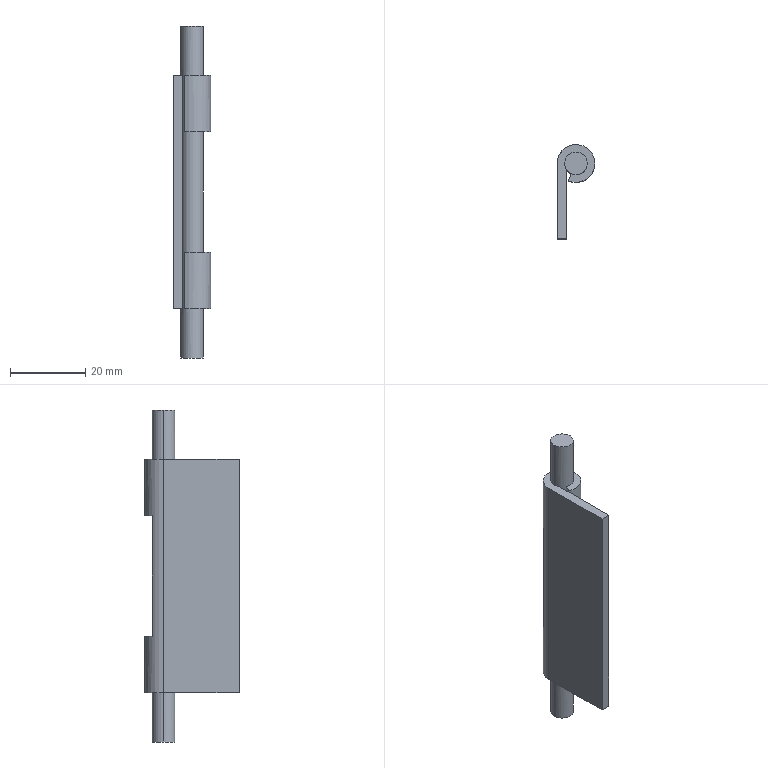Part | NX | features solid 2 | 1 solid | 17 faces | box 10 x 25 x 88 mm | volume 6948 mm3 | plane 12 | cylinder 5 | commonest cylinder face diameters 6 x4 10 x1
STEP:
#1=CARTESIAN_POINT('',(-1100.5,-763.,948.5));
#2=VERTEX_POINT('',#1);
#3=CARTESIAN_POINT('',(-1106.5,-763.,948.5));
#4=VERTEX_POINT('',#3);
#5=CARTESIAN_POINT('',(-1103.5,-763.,948.5));
#6=DIRECTION('',(0.,0.,-1.));
#7=DIRECTION('',(0.,1.,0.));
#8=AXIS2_PLACEMENT_3D('',#5,#6,#7);
#9=CIRCLE('',#8,3.);
#10=EDGE_CURVE('',#2,#4,#9,.T.);
#11=ORIENTED_EDGE('',*,*,#10,.F.);
#12=CARTESIAN_POINT('',(-1103.5,-763.,948.5));
#13=DIRECTION('',(0.,0.,-1.));
#14=DIRECTION('',(0.,1.,0.));
#15=AXIS2_PLACEMENT_3D('',#12,#13,#14);
#16=CIRCLE('',#15,3.);
#17=EDGE_CURVE('',#4,#2,#16,.T.);
#18=ORIENTED_EDGE('',*,*,#17,.F.);
#19=EDGE_LOOP('',(#11,#18));
#20=FACE_BOUND('',#19,.T.);
#21=CARTESIAN_POINT('',(-1103.5,-763.,948.5));
#22=DIRECTION('',(0.,0.,-1.));
#23=DIRECTION('',(0.,-1.,0.));
#24=AXIS2_PLACEMENT_3D('',#21,#22,#23);
#25=PLANE('',#24);
#26=ADVANCED_FACE('',(#20),#25,.F.);
#27=CARTESIAN_POINT('',(-1100.5,-763.,860.5));
#28=VERTEX_POINT('',#27);
#29=CARTESIAN_POINT('',(-1106.5,-763.,860.5));
#30=VERTEX_POINT('',#29);
#31=CARTESIAN_POINT('',(-1103.5,-763.,860.5));
#32=DIRECTION('',(0.,0.,-1.));
#33=DIRECTION('',(0.,1.,0.));
#34=AXIS2_PLACEMENT_3D('',#31,#32,#33);
#35=CIRCLE('',#34,3.);
#36=EDGE_CURVE('',#28,#30,#35,.T.);
#37=ORIENTED_EDGE('',*,*,#36,.T.);
#38=CARTESIAN_POINT('',(-1103.5,-763.,860.5));
#39=DIRECTION('',(0.,0.,-1.));
#40=DIRECTION('',(0.,1.,0.));
#41=AXIS2_PLACEMENT_3D('',#38,#39,#40);
#42=CIRCLE('',#41,3.);
#43=EDGE_CURVE('',#30,#28,#42,.T.);
#44=ORIENTED_EDGE('',*,*,#43,.T.);
#45=EDGE_LOOP('',(#37,#44));
#46=FACE_BOUND('',#45,.T.);
#47=CARTESIAN_POINT('',(-1103.5,-763.,860.5));
#48=DIRECTION('',(0.,0.,-1.));
#49=DIRECTION('',(0.,-1.,0.));
#50=AXIS2_PLACEMENT_3D('',#47,#48,#49);
#51=PLANE('',#50);
#52=ADVANCED_FACE('',(#46),#51,.T.);
#53=CARTESIAN_POINT('',(-1100.5,-763.,888.5));
#54=VERTEX_POINT('',#53);
#55=CARTESIAN_POINT('',(-1100.5,-763.,920.5));
#56=VERTEX_POINT('',#55);
#57=CARTESIAN_POINT('',(-1100.5,-763.,860.5));
#58=DIRECTION('',(0.,0.,1.));
#59=VECTOR('',#58,1000.);
#60=LINE('',#57,#59);
#61=EDGE_CURVE('',#54,#56,#60,.T.);
#62=ORIENTED_EDGE('',*,*,#61,.F.);
#63=CARTESIAN_POINT('',(-1105.9,-761.2,888.5));
#64=VERTEX_POINT('',#63);
#65=CARTESIAN_POINT('',(-1103.5,-763.,888.5));
#66=DIRECTION('',(0.,0.,1.));
#67=DIRECTION('',(1.,0.,0.));
#68=AXIS2_PLACEMENT_3D('',#65,#66,#67);
#69=CIRCLE('',#68,3.);
#70=EDGE_CURVE('',#54,#64,#69,.T.);
#71=ORIENTED_EDGE('',*,*,#70,.T.);
#72=CARTESIAN_POINT('',(-1105.9,-761.2,920.5));
#73=VERTEX_POINT('',#72);
#74=CARTESIAN_POINT('',(-1105.9,-761.2,860.5));
#75=DIRECTION('',(0.,0.,1.));
#76=VECTOR('',#75,1000.);
#77=LINE('',#74,#76);
#78=EDGE_CURVE('',#64,#73,#77,.T.);
#79=ORIENTED_EDGE('',*,*,#78,.T.);
#80=CARTESIAN_POINT('',(-1103.5,-763.,920.5));
#81=DIRECTION('',(0.,0.,-1.));
#82=DIRECTION('',(-1.,0.,0.));
#83=AXIS2_PLACEMENT_3D('',#80,#81,#82);
#84=CIRCLE('',#83,3.);
#85=EDGE_CURVE('',#73,#56,#84,.T.);
#86=ORIENTED_EDGE('',*,*,#85,.T.);
#87=EDGE_LOOP('',(#62,#71,#79,#86));
#88=FACE_BOUND('',#87,.T.);
#89=CARTESIAN_POINT('',(-1103.5,-763.,860.5));
#90=DIRECTION('',(0.,0.,1.));
#91=DIRECTION('',(1.,0.,0.));
#92=AXIS2_PLACEMENT_3D('',#89,#90,#91);
#93=CYLINDRICAL_SURFACE('',#92,3.);
#94=ADVANCED_FACE('',(#88),#93,.T.);
#95=CARTESIAN_POINT('',(-1106.,-783.,935.5));
#96=VERTEX_POINT('',#95);
#97=CARTESIAN_POINT('',(-1106.,-783.,873.5));
#98=VERTEX_POINT('',#97);
#99=CARTESIAN_POINT('',(-1106.,-783.,935.5));
#100=DIRECTION('',(0.,0.,-1.));
#101=VECTOR('',#100,1000.);
#102=LINE('',#99,#101);
#103=EDGE_CURVE('',#96,#98,#102,.T.);
#104=ORIENTED_EDGE('',*,*,#103,.F.);
#105=CARTESIAN_POINT('',(-1108.5,-783.,935.5));
#106=VERTEX_POINT('',#105);
#107=CARTESIAN_POINT('',(-1108.5,-783.,935.5));
#108=DIRECTION('',(-1.,0.,0.));
#109=VECTOR('',#108,1000.);
#110=LINE('',#107,#109);
#111=EDGE_CURVE('',#96,#106,#110,.T.);
#112=ORIENTED_EDGE('',*,*,#111,.T.);
#113=CARTESIAN_POINT('',(-1108.5,-783.,873.5));
#114=VERTEX_POINT('',#113);
#115=CARTESIAN_POINT('',(-1108.5,-783.,935.5));
#116=DIRECTION('',(0.,0.,-1.));
#117=VECTOR('',#116,1000.);
#118=LINE('',#115,#117);
#119=EDGE_CURVE('',#106,#114,#118,.T.);
#120=ORIENTED_EDGE('',*,*,#119,.T.);
#121=CARTESIAN_POINT('',(-1108.5,-783.,873.5));
#122=DIRECTION('',(-1.,0.,0.));
#123=VECTOR('',#122,1000.);
#124=LINE('',#121,#123);
#125=EDGE_CURVE('',#98,#114,#124,.T.);
#126=ORIENTED_EDGE('',*,*,#125,.F.);
#127=EDGE_LOOP('',(#104,#112,#120,#126));
#128=FACE_BOUND('',#127,.T.);
#129=CARTESIAN_POINT('',(-1108.5,-783.,935.5));
#130=DIRECTION('',(0.,1.,0.));
#131=DIRECTION('',(0.,0.,-1.));
#132=AXIS2_PLACEMENT_3D('',#129,#130,#131);
#133=PLANE('',#132);
#134=ADVANCED_FACE('',(#128),#133,.F.);
#135=CARTESIAN_POINT('',(-1105.5,-767.583,888.5));
#136=VERTEX_POINT('',#135);
#137=CARTESIAN_POINT('',(-1107.5,-760.,888.5));
#138=VERTEX_POINT('',#137);
#139=CARTESIAN_POINT('',(-1103.5,-763.,888.5));
#140=DIRECTION('',(0.,0.,1.));
#141=DIRECTION('',(-1.,0.,0.));
#142=AXIS2_PLACEMENT_3D('',#139,#140,#141);
#143=CIRCLE('',#142,5.);
#144=EDGE_CURVE('',#136,#138,#143,.T.);
#145=ORIENTED_EDGE('',*,*,#144,.F.);
#146=CARTESIAN_POINT('',(-1105.5,-767.583,873.5));
#147=VERTEX_POINT('',#146);
#148=CARTESIAN_POINT('',(-1105.5,-767.583,935.5));
#149=DIRECTION('',(0.,0.,-1.));
#150=VECTOR('',#149,1000.);
#151=LINE('',#148,#150);
#152=EDGE_CURVE('',#136,#147,#151,.T.);
#153=ORIENTED_EDGE('',*,*,#152,.T.);
#154=CARTESIAN_POINT('',(-1108.5,-763.,873.5));
#155=VERTEX_POINT('',#154);
#156=CARTESIAN_POINT('',(-1103.5,-763.,873.5));
#157=DIRECTION('',(0.,0.,-1.));
#158=DIRECTION('',(-1.,0.,0.));
#159=AXIS2_PLACEMENT_3D('',#156,#157,#158);
#160=CIRCLE('',#159,5.);
#161=EDGE_CURVE('',#155,#147,#160,.T.);
#162=ORIENTED_EDGE('',*,*,#161,.F.);
#163=CARTESIAN_POINT('',(-1108.5,-763.,935.5));
#164=VERTEX_POINT('',#163);
#165=CARTESIAN_POINT('',(-1108.5,-763.,935.5));
#166=DIRECTION('',(0.,0.,-1.));
#167=VECTOR('',#166,1000.);
#168=LINE('',#165,#167);
#169=EDGE_CURVE('',#164,#155,#168,.T.);
#170=ORIENTED_EDGE('',*,*,#169,.F.);
#171=CARTESIAN_POINT('',(-1105.5,-767.583,935.5));
#172=VERTEX_POINT('',#171);
#173=CARTESIAN_POINT('',(-1103.5,-763.,935.5));
#174=DIRECTION('',(0.,0.,-1.));
#175=DIRECTION('',(-1.,0.,0.));
#176=AXIS2_PLACEMENT_3D('',#173,#174,#175);
#177=CIRCLE('',#176,5.);
#178=EDGE_CURVE('',#164,#172,#177,.T.);
#179=ORIENTED_EDGE('',*,*,#178,.T.);
#180=CARTESIAN_POINT('',(-1105.5,-767.583,920.5));
#181=VERTEX_POINT('',#180);
#182=CARTESIAN_POINT('',(-1105.5,-767.583,935.5));
#183=DIRECTION('',(0.,0.,-1.));
#184=VECTOR('',#183,1000.);
#185=LINE('',#182,#184);
#186=EDGE_CURVE('',#172,#181,#185,.T.);
#187=ORIENTED_EDGE('',*,*,#186,.T.);
#188=CARTESIAN_POINT('',(-1107.5,-760.,920.5));
#189=VERTEX_POINT('',#188);
#190=CARTESIAN_POINT('',(-1103.5,-763.,920.5));
#191=DIRECTION('',(0.,0.,-1.));
#192=DIRECTION('',(1.,0.,0.));
#193=AXIS2_PLACEMENT_3D('',#190,#191,#192);
#194=CIRCLE('',#193,5.);
#195=EDGE_CURVE('',#189,#181,#194,.T.);
#196=ORIENTED_EDGE('',*,*,#195,.F.);
#197=CARTESIAN_POINT('',(-1107.5,-760.,935.5));
#198=DIRECTION('',(0.,0.,1.));
#199=VECTOR('',#198,1000.);
#200=LINE('',#197,#199);
#201=EDGE_CURVE('',#138,#189,#200,.T.);
#202=ORIENTED_EDGE('',*,*,#201,.F.);
#203=EDGE_LOOP('',(#145,#153,#162,#170,#179,#187,#196,#202));
#204=FACE_BOUND('',#203,.T.);
#205=CARTESIAN_POINT('',(-1103.5,-763.,935.5));
#206=DIRECTION('',(0.,0.,-1.));
#207=DIRECTION('',(-1.,0.,0.));
#208=AXIS2_PLACEMENT_3D('',#205,#206,#207);
#209=CYLINDRICAL_SURFACE('',#208,5.);
#210=ADVANCED_FACE('',(#204),#209,.T.);
#211=CARTESIAN_POINT('',(-1108.5,-783.,873.5));
#212=DIRECTION('',(0.,1.,0.));
#213=VECTOR('',#212,1000.);
#214=LINE('',#211,#213);
#215=EDGE_CURVE('',#114,#155,#214,.T.);
#216=ORIENTED_EDGE('',*,*,#215,.F.);
#217=ORIENTED_EDGE('',*,*,#119,.F.);
#218=CARTESIAN_POINT('',(-1108.5,-783.,935.5));
#219=DIRECTION('',(0.,1.,0.));
#220=VECTOR('',#219,1000.);
#221=LINE('',#218,#220);
#222=EDGE_CURVE('',#106,#164,#221,.T.);
#223=ORIENTED_EDGE('',*,*,#222,.T.);
#224=ORIENTED_EDGE('',*,*,#169,.T.);
#225=EDGE_LOOP('',(#216,#217,#223,#224));
#226=FACE_BOUND('',#225,.T.);
#227=CARTESIAN_POINT('',(-1108.5,-783.,935.5));
#228=DIRECTION('',(-1.,0.,0.));
#229=DIRECTION('',(0.,1.,0.));
#230=AXIS2_PLACEMENT_3D('',#227,#228,#229);
#231=PLANE('',#230);
#232=ADVANCED_FACE('',(#226),#231,.T.);
#233=ORIENTED_EDGE('',*,*,#78,.F.);
#234=CARTESIAN_POINT('',(-1105.5,-761.5,888.5));
#235=DIRECTION('',(0.8,-0.6,0.));
#236=VECTOR('',#235,1000.);
#237=LINE('',#234,#236);
#238=EDGE_CURVE('',#138,#64,#237,.T.);
#239=ORIENTED_EDGE('',*,*,#238,.F.);
#240=ORIENTED_EDGE('',*,*,#201,.T.);
#241=CARTESIAN_POINT('',(-1105.5,-761.5,920.5));
#242=DIRECTION('',(0.8,-0.6,0.));
#243=VECTOR('',#242,1000.);
#244=LINE('',#241,#243);
#245=EDGE_CURVE('',#189,#73,#244,.T.);
#246=ORIENTED_EDGE('',*,*,#245,.T.);
#247=EDGE_LOOP('',(#233,#239,#240,#246));
#248=FACE_BOUND('',#247,.T.);
#249=CARTESIAN_POINT('',(-1105.5,-761.5,904.5));
#250=DIRECTION('',(0.6,0.8,0.));
#251=DIRECTION('',(0.,0.,-1.));
#252=AXIS2_PLACEMENT_3D('',#249,#250,#251);
#253=PLANE('',#252);
#254=ADVANCED_FACE('',(#248),#253,.T.);
#255=ORIENTED_EDGE('',*,*,#85,.F.);
#256=ORIENTED_EDGE('',*,*,#245,.F.);
#257=ORIENTED_EDGE('',*,*,#195,.T.);
#258=CARTESIAN_POINT('',(-1104.7,-765.75,920.5));
#259=VERTEX_POINT('',#258);
#260=CARTESIAN_POINT('',(-1105.5,-767.583,920.5));
#261=DIRECTION('',(-0.4,-0.9165,0.));
#262=VECTOR('',#261,1000.);
#263=LINE('',#260,#262);
#264=EDGE_CURVE('',#259,#181,#263,.T.);
#265=ORIENTED_EDGE('',*,*,#264,.F.);
#266=CARTESIAN_POINT('',(-1103.5,-763.,920.5));
#267=DIRECTION('',(0.,0.,-1.));
#268=DIRECTION('',(-1.,0.,0.));
#269=AXIS2_PLACEMENT_3D('',#266,#267,#268);
#270=CIRCLE('',#269,3.);
#271=EDGE_CURVE('',#56,#259,#270,.T.);
#272=ORIENTED_EDGE('',*,*,#271,.F.);
#273=EDGE_LOOP('',(#255,#256,#257,#265,#272));
#274=FACE_BOUND('',#273,.T.);
#275=CARTESIAN_POINT('',(-1103.5,-763.,920.5));
#276=DIRECTION('',(0.,0.,-1.));
#277=DIRECTION('',(0.,-1.,0.));
#278=AXIS2_PLACEMENT_3D('',#275,#276,#277);
#279=PLANE('',#278);
#280=ADVANCED_FACE('',(#274),#279,.T.);
#281=CARTESIAN_POINT('',(-1104.7,-765.75,888.5));
#282=VERTEX_POINT('',#281);
#283=CARTESIAN_POINT('',(-1103.5,-763.,888.5));
#284=DIRECTION('',(0.,0.,1.));
#285=DIRECTION('',(1.,0.,0.));
#286=AXIS2_PLACEMENT_3D('',#283,#284,#285);
#287=CIRCLE('',#286,3.);
#288=EDGE_CURVE('',#282,#54,#287,.T.);
#289=ORIENTED_EDGE('',*,*,#288,.F.);
#290=CARTESIAN_POINT('',(-1105.5,-767.583,888.5));
#291=DIRECTION('',(-0.4,-0.9165,0.));
#292=VECTOR('',#291,1000.);
#293=LINE('',#290,#292);
#294=EDGE_CURVE('',#282,#136,#293,.T.);
#295=ORIENTED_EDGE('',*,*,#294,.T.);
#296=ORIENTED_EDGE('',*,*,#144,.T.);
#297=ORIENTED_EDGE('',*,*,#238,.T.);
#298=ORIENTED_EDGE('',*,*,#70,.F.);
#299=EDGE_LOOP('',(#289,#295,#296,#297,#298));
#300=FACE_BOUND('',#299,.T.);
#301=CARTESIAN_POINT('',(-1103.5,-763.,888.5));
#302=DIRECTION('',(0.,0.,1.));
#303=DIRECTION('',(0.,-1.,0.));
#304=AXIS2_PLACEMENT_3D('',#301,#302,#303);
#305=PLANE('',#304);
#306=ADVANCED_FACE('',(#300),#305,.T.);
#307=CARTESIAN_POINT('',(-1106.,-764.658,935.5));
#308=VERTEX_POINT('',#307);
#309=CARTESIAN_POINT('',(-1106.,-764.658,873.5));
#310=VERTEX_POINT('',#309);
#311=CARTESIAN_POINT('',(-1106.,-764.658,860.5));
#312=DIRECTION('',(0.,0.,-1.));
#313=VECTOR('',#312,1000.);
#314=LINE('',#311,#313);
#315=EDGE_CURVE('',#308,#310,#314,.T.);
#316=ORIENTED_EDGE('',*,*,#315,.F.);
#317=CARTESIAN_POINT('',(-1106.,-783.,935.5));
#318=DIRECTION('',(0.,1.,0.));
#319=VECTOR('',#318,1000.);
#320=LINE('',#317,#319);
#321=EDGE_CURVE('',#96,#308,#320,.T.);
#322=ORIENTED_EDGE('',*,*,#321,.F.);
#323=ORIENTED_EDGE('',*,*,#103,.T.);
#324=CARTESIAN_POINT('',(-1106.,-783.,873.5));
#325=DIRECTION('',(0.,1.,0.));
#326=VECTOR('',#325,1000.);
#327=LINE('',#324,#326);
#328=EDGE_CURVE('',#98,#310,#327,.T.);
#329=ORIENTED_EDGE('',*,*,#328,.T.);
#330=EDGE_LOOP('',(#316,#322,#323,#329));
#331=FACE_BOUND('',#330,.T.);
#332=CARTESIAN_POINT('',(-1106.,-783.,935.5));
#333=DIRECTION('',(-1.,0.,0.));
#334=DIRECTION('',(0.,1.,0.));
#335=AXIS2_PLACEMENT_3D('',#332,#333,#334);
#336=PLANE('',#335);
#337=ADVANCED_FACE('',(#331),#336,.F.);
#338=CARTESIAN_POINT('',(-1104.7,-765.75,873.5));
#339=VERTEX_POINT('',#338);
#340=CARTESIAN_POINT('',(-1105.5,-767.583,873.5));
#341=DIRECTION('',(-0.4,-0.9165,0.));
#342=VECTOR('',#341,1000.);
#343=LINE('',#340,#342);
#344=EDGE_CURVE('',#339,#147,#343,.T.);
#345=ORIENTED_EDGE('',*,*,#344,.F.);
#346=CARTESIAN_POINT('',(-1100.5,-763.,873.5));
#347=VERTEX_POINT('',#346);
#348=CARTESIAN_POINT('',(-1103.5,-763.,873.5));
#349=DIRECTION('',(0.,0.,1.));
#350=DIRECTION('',(0.,-1.,0.));
#351=AXIS2_PLACEMENT_3D('',#348,#349,#350);
#352=CIRCLE('',#351,3.);
#353=EDGE_CURVE('',#339,#347,#352,.T.);
#354=ORIENTED_EDGE('',*,*,#353,.T.);
#355=CARTESIAN_POINT('',(-1106.5,-763.,873.5));
#356=VERTEX_POINT('',#355);
#357=CARTESIAN_POINT('',(-1103.5,-763.,873.5));
#358=DIRECTION('',(0.,0.,1.));
#359=DIRECTION('',(0.,-1.,0.));
#360=AXIS2_PLACEMENT_3D('',#357,#358,#359);
#361=CIRCLE('',#360,3.);
#362=EDGE_CURVE('',#347,#356,#361,.T.);
#363=ORIENTED_EDGE('',*,*,#362,.T.);
#364=CARTESIAN_POINT('',(-1103.5,-763.,873.5));
#365=DIRECTION('',(0.,0.,1.));
#366=DIRECTION('',(0.,-1.,0.));
#367=AXIS2_PLACEMENT_3D('',#364,#365,#366);
#368=CIRCLE('',#367,3.);
#369=EDGE_CURVE('',#356,#310,#368,.T.);
#370=ORIENTED_EDGE('',*,*,#369,.T.);
#371=ORIENTED_EDGE('',*,*,#328,.F.);
#372=ORIENTED_EDGE('',*,*,#125,.T.);
#373=ORIENTED_EDGE('',*,*,#215,.T.);
#374=ORIENTED_EDGE('',*,*,#161,.T.);
#375=EDGE_LOOP('',(#345,#354,#363,#370,#371,#372,#373,#374));
#376=FACE_BOUND('',#375,.T.);
#377=CARTESIAN_POINT('',(-1108.5,-783.,873.5));
#378=DIRECTION('',(0.,0.,1.));
#379=DIRECTION('',(0.,-1.,0.));
#380=AXIS2_PLACEMENT_3D('',#377,#378,#379);
#381=PLANE('',#380);
#382=ADVANCED_FACE('',(#376),#381,.F.);
#383=ORIENTED_EDGE('',*,*,#294,.F.);
#384=CARTESIAN_POINT('',(-1104.7,-765.75,860.5));
#385=DIRECTION('',(0.,0.,-1.));
#386=VECTOR('',#385,1000.);
#387=LINE('',#384,#386);
#388=EDGE_CURVE('',#282,#339,#387,.T.);
#389=ORIENTED_EDGE('',*,*,#388,.T.);
#390=ORIENTED_EDGE('',*,*,#344,.T.);
#391=ORIENTED_EDGE('',*,*,#152,.F.);
#392=EDGE_LOOP('',(#383,#389,#390,#391));
#393=FACE_BOUND('',#392,.T.);
#394=CARTESIAN_POINT('',(-1105.5,-767.583,904.5));
#395=DIRECTION('',(-0.9165,0.4,0.));
#396=DIRECTION('',(0.,0.,1.));
#397=AXIS2_PLACEMENT_3D('',#394,#395,#396);
#398=PLANE('',#397);
#399=ADVANCED_FACE('',(#393),#398,.T.);
#400=ORIENTED_EDGE('',*,*,#321,.T.);
#401=CARTESIAN_POINT('',(-1106.5,-763.,935.5));
#402=VERTEX_POINT('',#401);
#403=CARTESIAN_POINT('',(-1103.5,-763.,935.5));
#404=DIRECTION('',(0.,0.,-1.));
#405=DIRECTION('',(0.,-1.,0.));
#406=AXIS2_PLACEMENT_3D('',#403,#404,#405);
#407=CIRCLE('',#406,3.);
#408=EDGE_CURVE('',#308,#402,#407,.T.);
#409=ORIENTED_EDGE('',*,*,#408,.T.);
#410=CARTESIAN_POINT('',(-1100.5,-763.,935.5));
#411=VERTEX_POINT('',#410);
#412=CARTESIAN_POINT('',(-1103.5,-763.,935.5));
#413=DIRECTION('',(0.,0.,-1.));
#414=DIRECTION('',(0.,-1.,0.));
#415=AXIS2_PLACEMENT_3D('',#412,#413,#414);
#416=CIRCLE('',#415,3.);
#417=EDGE_CURVE('',#402,#411,#416,.T.);
#418=ORIENTED_EDGE('',*,*,#417,.T.);
#419=CARTESIAN_POINT('',(-1104.7,-765.75,935.5));
#420=VERTEX_POINT('',#419);
#421=CARTESIAN_POINT('',(-1103.5,-763.,935.5));
#422=DIRECTION('',(0.,0.,-1.));
#423=DIRECTION('',(0.,-1.,0.));
#424=AXIS2_PLACEMENT_3D('',#421,#422,#423);
#425=CIRCLE('',#424,3.);
#426=EDGE_CURVE('',#411,#420,#425,.T.);
#427=ORIENTED_EDGE('',*,*,#426,.T.);
#428=CARTESIAN_POINT('',(-1105.5,-767.583,935.5));
#429=DIRECTION('',(-0.4,-0.9165,0.));
#430=VECTOR('',#429,1000.);
#431=LINE('',#428,#430);
#432=EDGE_CURVE('',#420,#172,#431,.T.);
#433=ORIENTED_EDGE('',*,*,#432,.T.);
#434=ORIENTED_EDGE('',*,*,#178,.F.);
#435=ORIENTED_EDGE('',*,*,#222,.F.);
#436=ORIENTED_EDGE('',*,*,#111,.F.);
#437=EDGE_LOOP('',(#400,#409,#418,#427,#433,#434,#435,#436));
#438=FACE_BOUND('',#437,.T.);
#439=CARTESIAN_POINT('',(-1103.5,-763.,935.5));
#440=DIRECTION('',(0.,0.,1.));
#441=DIRECTION('',(0.,-1.,0.));
#442=AXIS2_PLACEMENT_3D('',#439,#440,#441);
#443=PLANE('',#442);
#444=ADVANCED_FACE('',(#438),#443,.T.);
#445=ORIENTED_EDGE('',*,*,#432,.F.);
#446=CARTESIAN_POINT('',(-1104.7,-765.75,860.5));
#447=DIRECTION('',(0.,0.,-1.));
#448=VECTOR('',#447,1000.);
#449=LINE('',#446,#448);
#450=EDGE_CURVE('',#420,#259,#449,.T.);
#451=ORIENTED_EDGE('',*,*,#450,.T.);
#452=ORIENTED_EDGE('',*,*,#264,.T.);
#453=ORIENTED_EDGE('',*,*,#186,.F.);
#454=EDGE_LOOP('',(#445,#451,#452,#453));
#455=FACE_BOUND('',#454,.T.);
#456=CARTESIAN_POINT('',(-1105.5,-767.583,904.5));
#457=DIRECTION('',(-0.9165,0.4,0.));
#458=DIRECTION('',(0.,0.,1.));
#459=AXIS2_PLACEMENT_3D('',#456,#457,#458);
#460=PLANE('',#459);
#461=ADVANCED_FACE('',(#455),#460,.T.);
#462=CARTESIAN_POINT('',(-1106.5,-763.,860.5));
#463=DIRECTION('',(0.,0.,1.));
#464=VECTOR('',#463,1000.);
#465=LINE('',#462,#464);
#466=EDGE_CURVE('',#30,#356,#465,.T.);
#467=ORIENTED_EDGE('',*,*,#466,.F.);
#468=ORIENTED_EDGE('',*,*,#36,.F.);
#469=CARTESIAN_POINT('',(-1100.5,-763.,860.5));
#470=DIRECTION('',(0.,0.,1.));
#471=VECTOR('',#470,1000.);
#472=LINE('',#469,#471);
#473=EDGE_CURVE('',#347,#28,#472,.F.);
#474=ORIENTED_EDGE('',*,*,#473,.F.);
#475=ORIENTED_EDGE('',*,*,#353,.F.);
#476=ORIENTED_EDGE('',*,*,#388,.F.);
#477=ORIENTED_EDGE('',*,*,#288,.T.);
#478=ORIENTED_EDGE('',*,*,#61,.T.);
#479=ORIENTED_EDGE('',*,*,#271,.T.);
#480=ORIENTED_EDGE('',*,*,#450,.F.);
#481=ORIENTED_EDGE('',*,*,#426,.F.);
#482=CARTESIAN_POINT('',(-1100.5,-763.,860.5));
#483=DIRECTION('',(0.,0.,1.));
#484=VECTOR('',#483,1000.);
#485=LINE('',#482,#484);
#486=EDGE_CURVE('',#2,#411,#485,.F.);
#487=ORIENTED_EDGE('',*,*,#486,.F.);
#488=ORIENTED_EDGE('',*,*,#10,.T.);
#489=CARTESIAN_POINT('',(-1106.5,-763.,860.5));
#490=DIRECTION('',(0.,0.,1.));
#491=VECTOR('',#490,1000.);
#492=LINE('',#489,#491);
#493=EDGE_CURVE('',#402,#4,#492,.T.);
#494=ORIENTED_EDGE('',*,*,#493,.F.);
#495=ORIENTED_EDGE('',*,*,#408,.F.);
#496=ORIENTED_EDGE('',*,*,#315,.T.);
#497=ORIENTED_EDGE('',*,*,#369,.F.);
#498=EDGE_LOOP('',(#467,#468,#474,#475,#476,#477,#478,#479,#480,#481,#487,#488,#494,#495,#496,#497));
#499=FACE_BOUND('',#498,.T.);
#500=CARTESIAN_POINT('',(-1103.5,-763.,860.5));
#501=DIRECTION('',(0.,0.,1.));
#502=DIRECTION('',(1.,0.,0.));
#503=AXIS2_PLACEMENT_3D('',#500,#501,#502);
#504=CYLINDRICAL_SURFACE('',#503,3.);
#505=ADVANCED_FACE('',(#499),#504,.T.);
#506=ORIENTED_EDGE('',*,*,#417,.F.);
#507=ORIENTED_EDGE('',*,*,#493,.T.);
#508=ORIENTED_EDGE('',*,*,#17,.T.);
#509=ORIENTED_EDGE('',*,*,#486,.T.);
#510=EDGE_LOOP('',(#506,#507,#508,#509));
#511=FACE_BOUND('',#510,.T.);
#512=CARTESIAN_POINT('',(-1103.5,-763.,860.5));
#513=DIRECTION('',(0.,0.,1.));
#514=DIRECTION('',(1.,0.,0.));
#515=AXIS2_PLACEMENT_3D('',#512,#513,#514);
#516=CYLINDRICAL_SURFACE('',#515,3.);
#517=ADVANCED_FACE('',(#511),#516,.T.);
#518=ORIENTED_EDGE('',*,*,#43,.F.);
#519=ORIENTED_EDGE('',*,*,#466,.T.);
#520=ORIENTED_EDGE('',*,*,#362,.F.);
#521=ORIENTED_EDGE('',*,*,#473,.T.);
#522=EDGE_LOOP('',(#518,#519,#520,#521));
#523=FACE_BOUND('',#522,.T.);
#524=CARTESIAN_POINT('',(-1103.5,-763.,860.5));
#525=DIRECTION('',(0.,0.,1.));
#526=DIRECTION('',(1.,0.,0.));
#527=AXIS2_PLACEMENT_3D('',#524,#525,#526);
#528=CYLINDRICAL_SURFACE('',#527,3.);
#529=ADVANCED_FACE('',(#523),#528,.T.);
#530=CLOSED_SHELL('',(#26,#52,#94,#134,#210,#232,#254,#280,#306,#337,#382,#399,#444,#461,#505,#517,#529));
#531=MANIFOLD_SOLID_BREP('',#530);
#532=(LENGTH_UNIT()NAMED_UNIT(*)SI_UNIT(.MILLI.,.METRE.));
#533=UNCERTAINTY_MEASURE_WITH_UNIT(LENGTH_MEASURE(0.00001),#532,'','');
#534=(NAMED_UNIT(*)PLANE_ANGLE_UNIT()SI_UNIT($,.RADIAN.));
#535=(NAMED_UNIT(*)SI_UNIT($,.STERADIAN.)SOLID_ANGLE_UNIT());
#536=(GEOMETRIC_REPRESENTATION_CONTEXT(3)GLOBAL_UNCERTAINTY_ASSIGNED_CONTEXT((#533))GLOBAL_UNIT_ASSIGNED_CONTEXT((#532,#534,#535))REPRESENTATION_CONTEXT('',''));
#537=ADVANCED_BREP_SHAPE_REPRESENTATION('',(#531),#536);